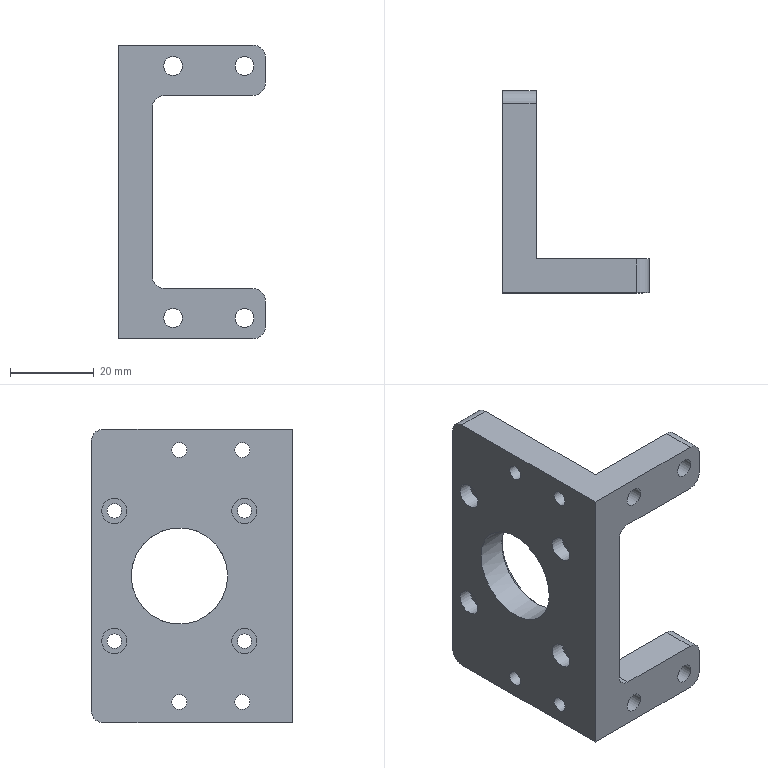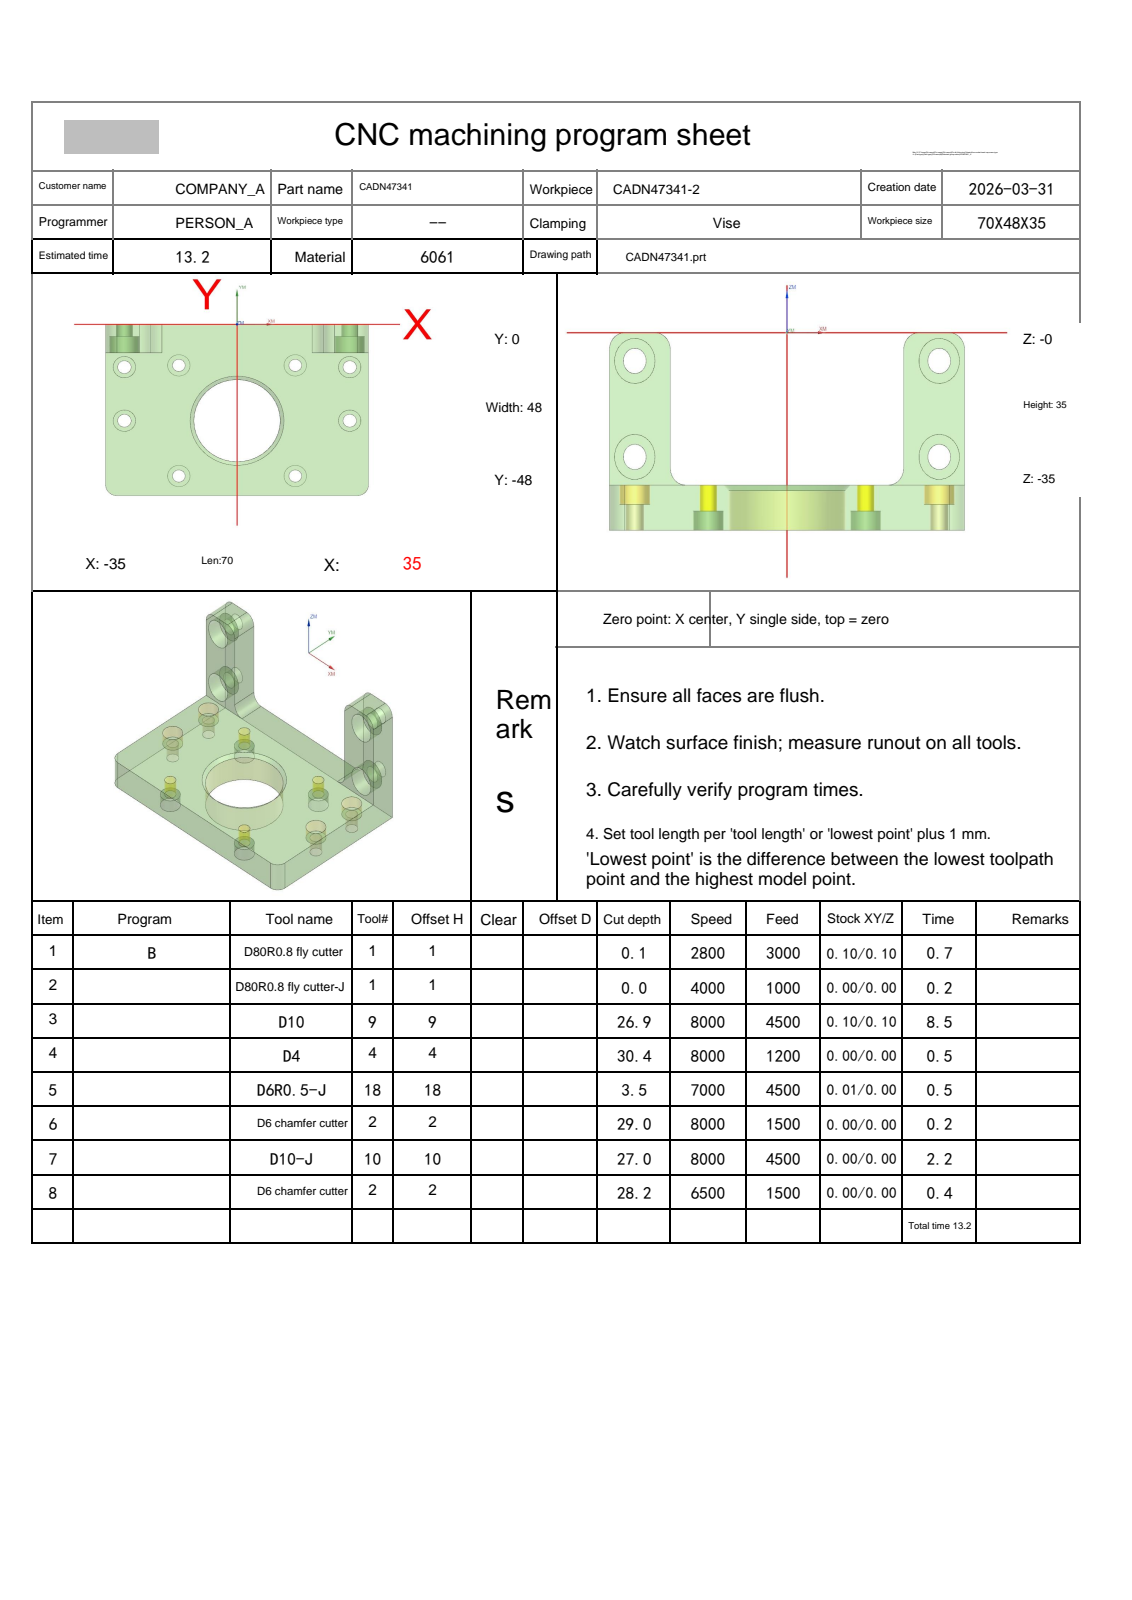NC program | NX | posted by the shop | part box 35 x 48 x 70 mm
Lines 8149 to 9805 of 13995:
N4 T04 M06
(D4  D=4. R=0. H=04 ce=0.07 di=0.00)
G00 G90 G54 X-30. Y-27. M03 S8000
G43 H04 Z20.
M08
Z-26.7
G03 X-30.465 Y-27.465 I0.0 J-.465 F1200.
X-30. Y-27.93 I.465 J0.0
X-30. Y-27.93 Z-26.9 I0.0 J.93
X-30. Y-27.93 Z-27.1 I0.0 J.93
X-30. Y-27.93 Z-27.3 I0.0 J.93
X-30. Y-27.93 Z-27.5 I0.0 J.93
X-30. Y-27.93 Z-27.7 I0.0 J.93
X-30. Y-27.93 Z-27.9 I0.0 J.93
X-30. Y-27.93 Z-28.1 I0.0 J.93
X-30. Y-27.93 Z-28.3 I0.0 J.93
X-30. Y-27.93 Z-28.5 I0.0 J.93
X-30. Y-27.93 Z-28.7 I0.0 J.93
X-30. Y-27.93 Z-28.9 I0.0 J.93
X-30. Y-27.93 Z-29.1 I0.0 J.93
X-30. Y-27.93 Z-29.3 I0.0 J.93
X-30. Y-27.93 Z-29.5 I0.0 J.93
X-30. Y-27.93 Z-29.7 I0.0 J.93
X-30. Y-27.93 Z-29.9 I0.0 J.93
X-30. Y-27.93 Z-30.1 I0.0 J.93
X-30. Y-27.93 Z-30.3 I0.0 J.93
X-30. Y-26.07 Z-30.4 I0.0 J.93
X-30.93 Y-27. I0.0 J-.93
X-30. Y-27.93 I.93 J0.0
X-29.07 Y-27. I0.0 J.93
X-30. Y-26.07 I-.93 J0.0
X-30.465 Y-26.535 I0.0 J-.465
X-30. Y-27. I.465 J0.0
G00 Z20.
Y-12.
Z-26.7
G03 X-30.465 Y-12.465 I0.0 J-.465
X-30. Y-12.93 I.465 J0.0
X-30. Y-12.93 Z-26.9 I0.0 J.93
X-30. Y-12.93 Z-27.1 I0.0 J.93
X-30. Y-12.93 Z-27.3 I0.0 J.93
X-30. Y-12.93 Z-27.5 I0.0 J.93
X-30. Y-12.93 Z-27.7 I0.0 J.93
X-30. Y-12.93 Z-27.9 I0.0 J.93
X-30. Y-12.93 Z-28.1 I0.0 J.93
X-30. Y-12.93 Z-28.3 I0.0 J.93
X-30. Y-12.93 Z-28.5 I0.0 J.93
X-30. Y-12.93 Z-28.7 I0.0 J.93
X-30. Y-12.93 Z-28.9 I0.0 J.93
X-30. Y-12.93 Z-29.1 I0.0 J.93
X-30. Y-12.93 Z-29.3 I0.0 J.93
X-30. Y-12.93 Z-29.5 I0.0 J.93
X-30. Y-12.93 Z-29.7 I0.0 J.93
X-30. Y-12.93 Z-29.9 I0.0 J.93
X-30. Y-12.93 Z-30.1 I0.0 J.93
X-30. Y-12.93 Z-30.3 I0.0 J.93
X-30. Y-11.07 Z-30.4 I0.0 J.93
X-30.93 Y-12. I0.0 J-.93
X-30. Y-12.93 I.93 J0.0
X-29.07 Y-12. I0.0 J.93
X-30. Y-11.07 I-.93 J0.0
X-30.465 Y-11.535 I0.0 J-.465
X-30. Y-12. I.465 J0.0
G00 Z20.
X30.
Z-26.7
G03 X29.535 Y-12.465 I0.0 J-.465
X30. Y-12.93 I.465 J0.0
X30. Y-12.93 Z-26.9 I0.0 J.93
X30. Y-12.93 Z-27.1 I0.0 J.93
X30. Y-12.93 Z-27.3 I0.0 J.93
X30. Y-12.93 Z-27.5 I0.0 J.93
X30. Y-12.93 Z-27.7 I0.0 J.93
X30. Y-12.93 Z-27.9 I0.0 J.93
X30. Y-12.93 Z-28.1 I0.0 J.93
X30. Y-12.93 Z-28.3 I0.0 J.93
X30. Y-12.93 Z-28.5 I0.0 J.93
X30. Y-12.93 Z-28.7 I0.0 J.93
X30. Y-12.93 Z-28.9 I0.0 J.93
X30. Y-12.93 Z-29.1 I0.0 J.93
X30. Y-12.93 Z-29.3 I0.0 J.93
X30. Y-12.93 Z-29.5 I0.0 J.93
X30. Y-12.93 Z-29.7 I0.0 J.93
X30. Y-12.93 Z-29.9 I0.0 J.93
X30. Y-12.93 Z-30.1 I0.0 J.93
X30. Y-12.93 Z-30.3 I0.0 J.93
X30. Y-11.07 Z-30.4 I0.0 J.93
X29.07 Y-12. I0.0 J-.93
X30. Y-12.93 I.93 J0.0
X30.93 Y-12. I0.0 J.93
X30. Y-11.07 I-.93 J0.0
X29.535 Y-11.535 I0.0 J-.465
X30. Y-12. I.465 J0.0
G00 Z20.
Y-27.
Z-26.7
G03 X29.535 Y-27.465 I0.0 J-.465
X30. Y-27.93 I.465 J0.0
X30. Y-27.93 Z-26.9 I0.0 J.93
X30. Y-27.93 Z-27.1 I0.0 J.93
X30. Y-27.93 Z-27.3 I0.0 J.93
X30. Y-27.93 Z-27.5 I0.0 J.93
X30. Y-27.93 Z-27.7 I0.0 J.93
X30. Y-27.93 Z-27.9 I0.0 J.93
X30. Y-27.93 Z-28.1 I0.0 J.93
X30. Y-27.93 Z-28.3 I0.0 J.93
X30. Y-27.93 Z-28.5 I0.0 J.93
X30. Y-27.93 Z-28.7 I0.0 J.93
X30. Y-27.93 Z-28.9 I0.0 J.93
X30. Y-27.93 Z-29.1 I0.0 J.93
X30. Y-27.93 Z-29.3 I0.0 J.93
X30. Y-27.93 Z-29.5 I0.0 J.93
X30. Y-27.93 Z-29.7 I0.0 J.93
X30. Y-27.93 Z-29.9 I0.0 J.93
X30. Y-27.93 Z-30.1 I0.0 J.93
X30. Y-27.93 Z-30.3 I0.0 J.93
X30. Y-26.07 Z-30.4 I0.0 J.93
X29.07 Y-27. I0.0 J-.93
X30. Y-27.93 I.93 J0.0
X30.93 Y-27. I0.0 J.93
X30. Y-26.07 I-.93 J0.0
X29.535 Y-26.535 I0.0 J-.465
X30. Y-27. I.465 J0.0
G00 Z20.
G00 G90 X-30. Y-27. M03 S8000
Z20.
Z-30.4
G01 X-30.272 Y-27.568 F600.
X-30.302 Y-27.698
G03 X-30. Y-28. I.302 J0.0
X-29. Y-27. I0.0 J1.
X-30. Y-26. I-1. J0.0
X-31. Y-27. I0.0 J-1.
X-30. Y-28. I1. J0.0
X-29.521 Y-27.878 I0.0 J1.
X-29.364 Y-27.613 I-.145 J.265
X-29.489 Y-27.368 I-.302 J0.0
G01 X-30. Y-27.
G00 Z20.
Y-12.
Z-30.4
G01 X-30.272 Y-12.568
X-30.302 Y-12.698
G03 X-30. Y-13. I.302 J0.0
X-29. Y-12. I0.0 J1.
X-30. Y-11. I-1. J0.0
X-31. Y-12. I0.0 J-1.
X-30. Y-13. I1. J0.0
X-29.521 Y-12.878 I0.0 J1.
X-29.364 Y-12.613 I-.145 J.265
X-29.489 Y-12.368 I-.302 J0.0
G01 X-30. Y-12.
G00 Z20.
X30.
Z-30.4
G01 X29.728 Y-12.568
X29.698 Y-12.698
G03 X30. Y-13. I.302 J0.0
X31. Y-12. I0.0 J1.
X30. Y-11. I-1. J0.0
X29. Y-12. I0.0 J-1.
X30. Y-13. I1. J0.0
X30.479 Y-12.878 I0.0 J1.
X30.636 Y-12.613 I-.145 J.265
X30.511 Y-12.368 I-.302 J0.0
G01 X30. Y-12.
G00 Z20.
Y-27.
Z-30.4
G01 X29.728 Y-27.568
X29.698 Y-27.698
G03 X30. Y-28. I.302 J0.0
X31. Y-27. I0.0 J1.
X30. Y-26. I-1. J0.0
X29. Y-27. I0.0 J-1.
X30. Y-28. I1. J0.0
X30.479 Y-27.878 I0.0 J1.
X30.636 Y-27.613 I-.145 J.265
X30.511 Y-27.368 I-.302 J0.0
G01 X30. Y-27.
G00 Z20.
G91 G28 Z0.0
M05
M09
G91 G28 Z0.0
M01
N5 T18 M06
(D6R0.5-J  D=6. R=0.5 H=18 ce=0.01 di=0.00)
G00 G90 G54 X34.089 Y6.274 M03 S7000
G43 H18 Z14.5
M08
Z.494
G01 Z-.006 F4500.
X34.596 Y1.122
X34.707 Y0.0
Y-8.
X34.606 Y-8.912
X34.546 Y-9.111
X34.648 Y-9.103 Z-.012
X34.682 Y-8.912
X34.794 Y-8.
Y0.0
X34.687 Y1.105
X34.742 Y1.101 Z-.015
X34.77 Y1.1 Z-.019
X34.877 Y0.0
Y-8.
X34.764 Y-8.912
X34.757 Y-9.1
X34.805 Z-.024
X34.838 Z-.03
X34.844 Y-8.912
X34.964 Y-8.
Y0.0
X34.848 Y1.1
X34.911 Z-.036
X34.942 Z-.042
X35.049 Y0.0
Y-8.
X34.939 Y-8.912
X34.935 Y-9.1
X35. Z-.049
X35.053 Z-.057
X35.056 Y-8.912
X35.138 Y-8.
Y0.0
X35.126 Y.048
X35.057 Y1.1
X35.109 Z-.066
X35.148 Z-.075
X35.208 Y.048
X35.228 Y0.0
Y-8.
X35.148 Y-8.912
X35.146 Y-9.1
X35.207 Z-.085
X35.241 Z-.095
X35.32 Y-8.
Y0.0
X35.302 Y.048
X35.243 Y1.1
X35.306 Z-.107
X35.351 Z-.118
X35.413 Y0.0
Y-8.
X35.349 Y-9.1
X35.406 Z-.132
X35.453 Z-.145
X35.456 Y-8.912
X35.506 Y-8.
Y0.0
X35.494 Y.048
X35.455 Y1.1
X35.504 Z-.159
X35.542 Z-.174
X35.583 Y.048
X35.598 Y0.0
Y-8.
X35.54 Y-9.1
X35.6 Z-.189
X35.635 Z-.205
X35.691 Y-8.
Y0.0
X35.68 Y.048
X35.637 Y1.1
X35.696 Z-.222
X35.74 Z-.24
X35.783 Y0.0
Y-8.
X35.741 Y-8.912
X35.738 Y-9.1
X35.791 Z-.258
X35.827 Z-.277
X35.874 Y-8.
Y0.0
X35.863 Y.048
X35.829 Y1.1
X35.883 Z-.297
X35.916 Z-.316
X35.964 Y0.0
Y-8.
X35.915 Y-9.1
X35.976 Z-.338
X36.008 Z-.359
X36.054 Y-8.
Y0.0
X36.01 Y1.1
X36.067 Z-.381
X36.109 Z-.404
X36.138 Y.048
X36.142 Y0.0
Y-8.
X36.108 Y-9.1
X36.155 Z-.427
X36.196 Z-.451
X36.229 Y-8.
Y0.0
X36.218 Y.048
X36.197 Y1.1
X36.244 Y1.101 Z-.476
X36.287 Z-.501
X36.304 Y.048
X36.315 Y0.0
Y-8.
X36.287 Y-9.1
X36.33 Z-.527
X36.369 Z-.554
X36.399 Y-8.
Y0.0
X36.393 Y.048
X36.37 Y1.1
X36.415 Z-.581
X36.456 Z-.609
X36.482 Y0.0
Y-8.
X36.454 Y-9.1
X36.499 Z-.637
X36.529 Z-.666
X36.564 Y-8.
Y0.0
X36.531 Y1.1
X36.58 Z-.696
X36.609 Z-.725
X36.632 Y.048
X36.643 Y0.0
Y-8.
X36.61 Y-8.912
X36.607 Y-9.1
X36.659 Z-.756
X36.688 Z-.787
X36.722 Y-8.
Y0.0
X36.69 Y1.1
X36.737 Z-.819
X36.774 Z-.851
X36.793 Y.171
X36.798 Y0.0
Y-8.
X36.772 Y-9.1
X36.814 Z-.884
X36.848 Z-.918
X36.872 Y-8.
Y0.0
X36.849 Y1.1
X36.888 Z-.952
X36.924 Z-.986
X36.945 Y0.0
Y-8.
X36.923 Y-9.1
X36.96 Z-1.021
X36.994 Z-1.056
X37.016 Y-8.
Y0.0
X36.995 Y1.1
X37.031 Z-1.093
X37.063 Z-1.129
X37.085 Y0.0
Y-8.
X37.061 Y-9.1
X37.098 Z-1.166
X37.13 Z-1.203
X37.151 Y-8.
Y0.0
X37.132 Y1.1
X37.167 Z-1.241
X37.193 Z-1.28
X37.216 Y0.0
Y-8.
X37.194 Y-8.912
X37.192 Y-9.1
X37.229 Z-1.319
X37.255 Z-1.358
X37.257 Y-8.912
X37.278 Y-8.
Y0.0
X37.256 Y1.1
X37.29 Z-1.398
X37.318 Z-1.438
X37.335 Y.048
X37.338 Y0.0
Y-8.
X37.319 Y-8.912
X37.317 Y-9.1
X37.349 Z-1.478
X37.372 Z-1.519
X37.371 Y-8.937
G02 X37.396 Y-8. I18.046 J0.0
G01 Y0.0
X37.391 Y.048
X37.373 Y1.1
X37.407 Z-1.561
X37.43 Z-1.602
X37.448 Y.048
X37.451 Y0.0
Y-8.
G03 X37.428 Y-8.963 I20.006 J-.963
G01 Y-9.1
X37.46 Z-1.645
X37.484 Z-1.687
Y-8.956
G02 X37.504 Y-8. I22.687 J0.0
G01 Y0.0
X37.501 Y.048
X37.482 Y1.199
X37.525 Y1.254 Z-1.773
G03 X37.554 Y0.0 I77.48 J1.165
G01 Y-8.
G03 X37.531 Y-8.927 I18.186 J-.927
G01 X37.532 Y-9.1
X37.563 Z-1.817
X37.58 Z-1.861
X37.579 Y-8.943
G02 X37.603 Y-8. I19.076 J0.0
G01 Y0.0
G02 X37.573 Y1.254 I126.284 J3.571
G01 X37.605 Z-1.905
X37.622 Z-1.95
G02 X37.648 Y0.0 I-513.452 J-11.351
G01 Y-8.
G03 X37.629 Y-9.028 I27.301 J-1.028
G01 Y-9.1
X37.654 Z-1.995
X37.671 Z-2.04
X37.67 Y-8.92
G02 X37.691 Y-8. I19.851 J0.0
G01 Y0.0
G02 X37.666 Y1.254 I55.734 J1.76
G01 X37.691 Z-2.086
X37.703 Z-2.132
G03 X37.731 Y0.0 I31.796 J.092
G01 Y-8.
G03 X37.706 Y-8.904 I15.853 J-.904
G01 X37.707 Y-9.1
X37.735 Z-2.178
X37.744 Z-2.224
X37.743 Y-8.917
G02 X37.769 Y-8. I15.88 J0.0
G01 Y0.0
G02 X37.741 Y1.21 I25.837 J1.21
G01 Y1.254
X37.768 Z-2.271
X37.776 Z-2.318
G03 X37.804 Y0.0 I68.546 J.918
G01 Y-8.
G03 X37.781 Y-8.97 I19.819 J-.97
G01 Y-9.1
X37.804 Z-2.365
X37.821 Z-2.412
G02 X37.82 Y-8.869 I22.498 J.231
X37.837 Y-8. I22.499 J0.0
G01 Y0.0
X37.834 Y.048
X37.821 Y1.1
X37.836 Z-2.46
X37.85 Z-2.508
G03 X37.847 Y.791 I15.845 J-.309
X37.866 Y0.0 I15.848 J0.0
G01 Y-8.
G03 X37.845 Y-8.923 I19.458 J-.923
G01 Y-9.092
X37.871 Y-9.084 Z-2.604
Y-8.924
G02 X37.893 Y-8. I18.828 J0.0
G01 Y0.0
G02 X37.873 Y.741 I13.709 J.741
X37.878 Y1.102 I13.729 J0.0
G01 X37.892 Y1.101 Z-2.653
X37.902 Z-2.701
G03 X37.9 Y.82 I18.924 J-.281
X37.918 Y0.0 I18.926 J0.0
G01 Y-8.
G03 X37.898 Y-8.975 I23.649 J-.975
G01 Y-9.076
X37.921 Y-9.067 Z-2.799
Y-8.923
G02 X37.939 Y-8. I23.129 J0.0
G01 Y0.0
G02 X37.922 Y.854 I21.386 J.854
X37.923 Y1.1 I21.403 J0.0
G01 X37.93 Z-2.848
X37.945 Z-2.897
G03 X37.941 Y.744 I16.614 J-.356
X37.958 Y0.0 I16.618 J0.0
G01 Y-8.
G03 X37.939 Y-8.93 I22.724 J-.93
G01 Y-9.059
X37.957 Y-9.051 Z-2.996
Y-8.952
G02 X37.974 Y-8. I27.373 J0.0
G01 Y0.0
X37.958 Y1.095
X37.962 Z-3.046
X37.971 Y1.096 Z-3.095
X37.987 Y0.0
Y-8.
X37.974 Y-8.912
X37.972 Y-9.042
X37.986 Y-9.034 Z-3.195
X37.997 Y-8.
Y0.0
X37.992 Y.048
X37.981 Y1.096
X37.989 Y1.097 Z-3.271
X37.997 Y.048
X38.003 Y0.0
Y-8.
G03 X37.991 Y-8.832 I30.152 J-.832
G01 X37.992 Y-9.027
X37.998 Y-9.02 Z-3.347
X38.007 Y-8.
Y0.0
X38.001 Y.048
X37.996 Y1.097
X38.003 Y1.098 Z-3.424
X38.006 Y.048
X38.009 Y0.0
Y-8.
X38.004 Y-9.014
X38.009 Y-9.007 Z-3.5
X38.01 Y-8.912
Y-8.
Y0.0
Y1.098
G00 Z14.5
X23.1 Y-13.856
Z.494
G01 Z-.006
X23.4 Y-9.1
X23.399 Y-8.912
X23.293 Y-8.
Y0.0
G03 X23.405 Y.947 I-3.948 J.947
G01 X23.402 Y1.1
X23.352 Z-.009
X23.344 Z-.012
X23.345 Y1.025
G02 X23.206 Y0.0 I-3.853 J0.0
G01 Y-8.
X23.338 Y-8.912
X23.34 Y-9.1
X23.261 Z-.019
X23.259 Y-8.912
X23.123 Y-8.
Y0.0
X23.269 Y1.1
X23.194 Z-.024
X23.17 Z-.03
X23.036 Y0.0
Y-8.
X23.158 Y-9.1
X23.089 Z-.036
X23.054 Z-.042
X23.053 Y-8.912
X22.951 Y-8.
Y0.0
X22.976 Y.048
X23.063 Y1.1
X23. Z-.049
X22.974 Z-.057
X22.887 Y.048
X22.862 Y0.0
Y-8.
X22.967 Y-8.912
X22.969 Y-9.1
X22.889 Z-.066
X22.869 Z-.075
X22.866 Y-8.912
X22.772 Y-8.
Y0.0
X22.781 Y.048
X22.869 Y1.1
X22.794 Z-.085
X22.75 Z-.095
X22.69 Y.048
X22.68 Y0.0
Y-8.
X22.749 Y-8.912
X22.752 Y-9.1
X22.694 Z-.107
X22.662 Z-.118
X22.587 Y-8.
Y0.0
X22.661 Y1.1
X22.592 Z-.132
X22.565 Z-.145
X22.494 Y0.0
Y-8.
X22.567 Y-9.1
X22.496 Z-.159
X22.461 Z-.174
X22.459 Y-8.912
X22.402 Y-8.
Y0.0
X22.46 Y1.1
X22.4 Z-.189
X22.359 Z-.205
X22.319 Y.048
X22.309 Y0.0
Y-8.
X22.36 Y-9.1
X22.303 Z-.222
X22.271 Z-.24
X22.217 Y-8.
Y0.0
X22.231 Y.048
X22.27 Y1.1
X22.209 Z-.258
X22.174 Z-.277
X22.136 Y.048
X22.126 Y0.0
Y-8.
X22.175 Y-9.1
X22.117 Z-.297
X22.072 Z-.316
X22.07 Y-8.912
X22.036 Y-8.
Y0.0
X22.071 Y1.1
X22.024 Z-.338
X21.985 Z-.359
X21.957 Y.048
X21.946 Y0.0
Y-8.
X21.986 Y-9.1
X21.933 Z-.381
X21.9 Z-.404
X21.858 Y-8.
Y0.0
X21.87 Y.048
X21.899 Y1.1
X21.845 Z-.427
X21.808 Z-.451
X21.778 Y.048
X21.771 Y0.0
Y-8.
X21.81 Y-9.1
X21.757 Z-.476
X21.714 Z-.501
X21.685 Y-8.
Y0.0
X21.712 Y1.1
X21.67 Z-.527
X21.635 Z-.554
X21.601 Y0.0
Y-8.
X21.636 Y-9.1
X21.585 Z-.581
X21.556 Z-.609
X21.554 Y-8.912
X21.518 Y-8.
Y0.0
X21.554 Y1.1
X21.501 Z-.637
X21.47 Z-.666
X21.436 Y0.0
Y-8.
X21.472 Y-9.1
X21.42 Z-.696
X21.385 Z-.725
X21.357 Y-8.
Y0.0
X21.384 Y1.1
X21.341 Z-.756
X21.309 Z-.787
X21.282 Y.048
X21.278 Y0.0
Y-8.
X21.308 Y-8.912
X21.31 Y-9.1
X21.262 Z-.819
X21.236 Z-.851
X21.234 Y-8.912
X21.202 Y-8.
Y0.0
G03 X21.237 Y.905 I-11.878 J.905
G01 X21.235 Y1.1
X21.186 Z-.884
X21.159 Z-.918
X21.131 Y.048
X21.128 Y0.0
Y-8.
X21.158 Y-8.912
X21.16 Y-9.1
X21.112 Z-.952
X21.081 Z-.986
X21.055 Y-8.
Y0.0
X21.08 Y1.1
X21.04 Z-1.021
X21.004 Z-1.056
X20.984 Y0.0
Y-8.
X21.005 Y-9.1
X20.969 Z-1.093
X20.938 Z-1.129
X20.915 Y-8.
Y0.0
X20.937 Y1.1
X20.902 Z-1.166
X20.868 Z-1.203
X20.849 Y0.0
Y-8.
X20.87 Y-9.1
X20.835 Z-1.241
X20.807 Z-1.28
X20.805 Y-8.912
X20.784 Y-8.
Y0.0
X20.806 Y1.1
X20.771 Z-1.319
X20.744 Z-1.358
X20.722 Y0.0
Y-8.
X20.743 Y-8.912
X20.745 Y-9.1
X20.71 Z-1.398
X20.681 Z-1.438
X20.68 Y-8.912
X20.662 Y-8.
Y0.0
X20.68 Y1.1
X20.648 Z-1.478
X20.626 Z-1.519
X20.609 Y.048
X20.604 Y0.0
Y-8.
G02 X20.628 Y-8.94 I-18.759 J-.94
G01 X20.627 Y-9.1
X20.594 Z-1.561
X20.572 Z-1.602
Y-8.956
G03 X20.549 Y-8. I-19.736 J0.0
G01 Y0.0
X20.552 Y.048
X20.57 Y1.1
X20.54 Y1.101 Z-1.645
X20.514 Z-1.687
X20.498 Y.048
X20.496 Y0.0
Y-8.
X20.513 Y-8.912
X20.515 Y-9.1
X20.485 Z-1.73
X20.467 Z-1.773
X20.468 Y-8.935
G03 X20.446 Y-8. I-19.449 J0.0
G01 Y0.0
X20.451 Y.048
X20.466 Y1.1
X20.438 Z-1.817
X20.419 Z-1.861
X20.403 Y.048
X20.397 Y0.0
Y-8.
G02 X20.42 Y-8.942 I-19.368 J-.942
G01 Y-9.1
X20.391 Z-1.905
X20.371 Z-1.95
G03 X20.352 Y-8. I-115.458 J-1.499
G01 Y0.0
X20.354 Y.048
X20.37 Y1.1
X20.347 Z-1.995
X20.324 Z-2.04
G02 X20.326 Y.872 I-22.983 J-.227
X20.309 Y0.0 I-22.984 J0.0
G01 Y-8.
G02 X20.326 Y-8.946 I-25.592 J-.946
G01 Y-9.1
X20.303 Z-2.086
X20.287 Z-2.132
G03 X20.289 Y-8.886 I-19.68 J.214
X20.269 Y-8. I-19.681 J0.0
G01 Y0.0
G03 X20.288 Y.808 I-16.637 J.808
X20.286 Y1.1 I-16.657 J0.0
G01 X20.265 Z-2.178
X20.247 Z-2.224
G02 X20.251 Y.778 I-15.101 J-.322
X20.231 Y0.0 I-15.104 J0.0
G01 Y-8.
G02 X20.251 Y-8.815 I-16.022 J-.815
X20.249 Y-9.1 I-16.043 J0.0
G01 X20.229 Z-2.271
X20.216 Z-2.318
X20.217 Y-8.905
G03 X20.196 Y-8. I-19.286 J0.0
G01 Y0.0
G03 X20.216 Y.827 I-16.483 J.827
X20.214 Y1.1 I-16.504 J0.0
G01 X20.195 Z-2.365
X20.181 Z-2.412
Y.915
G02 X20.163 Y0.0 I-23.204 J0.0
G01 Y-8.
G02 X20.183 Y-9.015 I-26.535 J-1.015
G01 Y-9.101
X20.164 Z-2.46
X20.153 Z-2.508
X20.154 Y-8.937
G03 X20.134 Y-8. I-21.378 J0.0
G01 Y0.0
G03 X20.153 Y.892 I-20.57 J.892
X20.152 Y1.1 I-20.589 J0.0
G01 X20.133 Z-2.556
X20.126 Z-2.604
G02 X20.128 Y.896 I-19.123 J-.205
X20.107 Y0.0 I-19.124 J0.0
G01 Y-8.
G02 X20.129 Y-8.943 I-19.919 J-.943
G01 X20.128 Y-9.101
X20.111 Z-2.653
X20.103 Z-2.701
Y-8.999
G03 X20.082 Y-8. I-24.126 J0.0
G01 Y0.0
G03 X20.102 Y.929 I-22.514 J.929
G01 X20.101 Y1.1
X20.087 Z-2.75
X20.077 Z-2.799
X20.078 Y.902
G02 X20.061 Y0.0 I-24.129 J0.0
G01 Y-8.
G02 X20.079 Y-8.969 I-26.133 J-.969
G01 Y-9.1
X20.07 Y-9.101 Z-2.848
X20.062 Z-2.897
Y-9.066
G03 X20.042 Y-8. I-29.214 J0.0
G01 Y0.0
G03 X20.06 Y.913 I-23.599 J.912
G01 X20.059 Y1.1
X20.052 Z-2.947
X20.041 Y1.101 Z-2.996
X20.03 Y.048
X20.026 Y0.0
Y-8.
X20.045 Y-9.101
X20.035 Y-9.1 Z-3.046
X20.032 Z-3.095
Y-8.992
G03 X20.013 Y-8. I-26.764 J0.0
G01 Y0.0
X20.019 Y.048
X20.029 Y1.1
X20.02 Z-3.145
X20.018 Z-3.195
G02 X20.02 Y.838 I-21.327 J-.262
X20.003 Y0.0 I-21.329 J0.0
G01 Y-8.
X20.021 Y-9.1
X20.013 Z-3.271
X19.998 Y-8.
Y0.0
G03 X20.011 Y.841 I-26.074 J.841
X20.01 Y1.1 I-26.088 J0.0
G01 X20.001 Z-3.347
X19.993 Y0.0
Y-8.
X20.005 Y-9.1
X19.995 Y-9.097 Z-3.424
X19.991 Y-8.
Y0.0
X19.994 Y1.099
X19.99 Y1.098 Z-3.5
Y0.0
Y-8.
Y-8.912
X19.992 Y-9.085
G00 Z14.5
X-23.167 Y5.901
Z.494
G01 Z-.006
X-23.399 Y1.1
X-23.404 Y.914
G03 X-23.293 Y0.0 I3.836 J0.0
G01 Y-8.
X-23.404 Y-9.1
X-23.352 Z-.009
X-23.345 Z-.012
X-23.206 Y-8.
Y0.0
G02 X-23.341 Y.96 I3.347 J.96
G01 X-23.338 Y1.1
X-23.259 Z-.019
X-23.123 Y0.0
Y-8.
X-23.27 Y-9.1
X-23.193 Z-.024
X-23.171 Z-.03
X-23.036 Y-8.
Y0.0
X-23.156 Y1.1
X-23.089 Z-.036
X-23.053 Z-.042
X-22.951 Y0.0
Y-8.
X-23.061 Y-8.912
X-23.064 Y-9.1
X-23. Z-.049
X-22.976 Z-.057
X-22.973 Y-8.912
X-22.862 Y-8.
Y0.0
X-22.968 Y1.1
X-22.89 Z-.066
X-22.867 Z-.075
X-22.772 Y0.0
Y-8.
X-22.872 Y-9.1
X-22.794 Z-.085
X-22.752 Z-.095
X-22.749 Y-8.912
X-22.68 Y-8.
Y0.0
X-22.69 Y.048
X-22.75 Y1.1
X-22.694 Z-.107
X-22.661 Z-.118
X-22.587 Y0.0
Y-8.
X-22.662 Y-9.1
X-22.592 Z-.132
X-22.567 Z-.145
X-22.494 Y-8.
Y0.0
X-22.565 Y1.1
X-22.496 Z-.159
X-22.46 Z-.174
X-22.402 Y0.0
Y-8.
X-22.459 Y-8.912
X-22.461 Y-9.1
X-22.4 Z-.189
X-22.36 Z-.205
X-22.309 Y-8.
Y0.0
X-22.319 Y.048
X-22.359 Y1.1
X-22.303 Z-.222
X-22.27 Z-.24
X-22.231 Y.048
X-22.217 Y0.0
Y-8.
X-22.271 Y-9.1
X-22.209 Z-.258
X-22.175 Z-.277
X-22.126 Y-8.
Y0.0
X-22.136 Y.048
X-22.174 Y1.1
X-22.117 Z-.297
X-22.071 Z-.316
X-22.036 Y0.0
Y-8.
X-22.07 Y-8.912
X-22.072 Y-9.1
X-22.024 Z-.338
X-21.986 Z-.359
X-21.946 Y-8.
Y0.0
X-21.957 Y.048
X-21.985 Y1.1
X-21.933 Z-.381
X-21.899 Z-.404
X-21.87 Y.048
X-21.858 Y0.0
Y-8.
X-21.9 Y-9.1
X-21.845 Z-.427
X-21.81 Z-.451
X-21.771 Y-8.
Y0.0
X-21.778 Y.048
X-21.808 Y1.1
X-21.757 Z-.476
X-21.712 Z-.501
X-21.688 Y.048
X-21.685 Y0.0
Y-8.
X-21.714 Y-9.1
X-21.67 Z-.527
X-21.636 Z-.554
X-21.601 Y-8.
Y0.0
X-21.635 Y1.1
X-21.585 Z-.581
X-21.554 Z-.609
X-21.518 Y0.0
Y-8.
X-21.554 Y-8.912
X-21.556 Y-9.1
X-21.501 Z-.637
X-21.472 Z-.666
X-21.436 Y-8.
Y0.0
X-21.47 Y1.1
X-21.42 Z-.696
X-21.384 Z-.725
X-21.357 Y0.0
Y-8.
X-21.385 Y-9.1
X-21.341 Z-.756
X-21.31 Z-.787
X-21.308 Y-8.912
X-21.278 Y-8.
Y0.0
X-21.282 Y.048
X-21.309 Y1.1
X-21.262 Z-.819
X-21.235 Z-.851
X-21.237 Y.905
G03 X-21.202 Y0.0 I11.913 J0.0
G01 Y-8.
X-21.234 Y-8.912
X-21.236 Y-9.1
X-21.186 Z-.884
X-21.16 Z-.918
X-21.158 Y-8.912
X-21.128 Y-8.
Y0.0
X-21.131 Y.048
X-21.159 Y1.1
X-21.112 Z-.952
X-21.08 Z-.986
X-21.055 Y0.0
Y-8.
X-21.081 Y-9.1
X-21.04 Z-1.021
X-21.005 Z-1.056
X-20.984 Y-8.
Y0.0
X-21.004 Y1.1
X-20.969 Z-1.093
X-20.937 Z-1.129
X-20.915 Y0.0
Y-8.
X-20.938 Y-9.1
X-20.902 Z-1.166
X-20.87 Z-1.203
X-20.849 Y-8.
Y0.0
X-20.868 Y1.1
X-20.835 Z-1.241
X-20.806 Z-1.28
X-20.784 Y0.0
Y-8.
X-20.805 Y-8.912
X-20.807 Y-9.1
X-20.771 Z-1.319
X-20.745 Z-1.358
X-20.743 Y-8.912
X-20.722 Y-8.
Y0.0
X-20.744 Y1.1
X-20.71 Z-1.398
X-20.68 Z-1.438
X-20.662 Y0.0
Y-8.
X-20.68 Y-8.912
X-20.681 Y-9.1
X-20.651 Z-1.478
X-20.627 Z-1.519
X-20.628 Y-8.94
G02 X-20.604 Y-8. I18.782 J0.0
G01 Y0.0
X-20.609 Y.048
X-20.626 Y1.1
X-20.593 Z-1.561
X-20.57 Z-1.602
X-20.552 Y.048
X-20.549 Y0.0
Y-8.
G03 X-20.572 Y-8.956 I19.712 J-.956
G01 Y-9.1
X-20.54 Z-1.645
X-20.515 Z-1.687
X-20.513 Y-8.912
X-20.496 Y-8.
Y0.0
X-20.514 Y1.101
X-20.487 Z-1.73
X-20.466 Y1.1 Z-1.773
X-20.451 Y.048
X-20.446 Y0.0
Y-8.
G03 X-20.468 Y-8.935 I19.427 J-.935
G01 X-20.467 Y-9.1
X-20.438 Z-1.817
X-20.42 Z-1.861
Y-8.942
G02 X-20.397 Y-8. I19.391 J0.0
G01 Y0.0
X-20.403 Y.048
X-20.419 Y1.1
X-20.391 Z-1.905
X-20.37 Z-1.95
X-20.354 Y.048
X-20.352 Y0.0
Y-8.
G03 X-20.372 Y-9.012 I26. J-1.011
G01 X-20.371 Y-9.1
X-20.347 Z-1.995
X-20.326 Z-2.04
Y-8.946
G02 X-20.309 Y-8. I25.61 J0.0
G01 Y0.0
G02 X-20.326 Y.872 I22.968 J.872
X-20.324 Y1.1 I22.984 J0.0
G01 X-20.305 Z-2.086
X-20.286 Z-2.132
G03 X-20.288 Y.808 I16.654 J-.291
X-20.269 Y0.0 I16.657 J0.0
G01 Y-8.
G03 X-20.289 Y-8.886 I19.661 J-.886
X-20.287 Y-9.1 I19.681 J0.0
G01 X-20.265 Z-2.178
X-20.249 Z-2.224
G02 X-20.251 Y-8.815 I16.04 J.285
X-20.231 Y-8. I16.043 J0.0
G01 Y0.0
G02 X-20.251 Y.778 I15.084 J.778
X-20.247 Y1.1 I15.104 J0.0
G01 X-20.229 Z-2.271
X-20.214 Z-2.318
G03 X-20.216 Y.827 I16.501 J-.273
X-20.196 Y0.0 I16.504 J0.0
G01 Y-8.
G03 X-20.217 Y-8.905 I19.264 J-.905
G01 X-20.216 Y-9.1
X-20.196 Z-2.365
X-20.183 Y-9.101 Z-2.412
Y-9.015
G02 X-20.163 Y-8. I26.554 J0.0
G01 Y0.0
G02 X-20.181 Y.915 I23.186 J.915
G01 Y1.1
X-20.164 Z-2.46
X-20.152 Z-2.508
G03 X-20.153 Y.892 I20.588 J-.207
X-20.134 Y0.0 I20.589 J0.0
G01 Y-8.
G03 X-20.154 Y-8.937 I21.357 J-.937
G01 X-20.153 Y-9.1
X-20.136 Y-9.101 Z-2.556
X-20.128 Z-2.604
X-20.129 Y-8.943
G02 X-20.107 Y-8. I19.94 J0.0
G01 Y0.0
G02 X-20.128 Y.896 I19.103 J.896
X-20.126 Y1.1 I19.124 J0.0
G01 X-20.108 Z-2.653
X-20.101 Z-2.701
X-20.102 Y.929
G03 X-20.082 Y0.0 I22.534 J0.0
G01 Y-8.
G03 X-20.103 Y-8.999 I24.104 J-.999
G01 Y-9.101
X-20.087 Z-2.75
X-20.078 Y-9.1 Z-2.799
X-20.079 Y-8.959
G02 X-20.061 Y-8. I25.656 J0.0
G01 Y0.0
G02 X-20.078 Y.913 I24.651 J.913
G01 X-20.077 Y1.1
X-20.07 Z-2.848
X-20.06 Z-2.897
Y.961
G03 X-20.042 Y0.0 I25.672 J0.0
G01 Y-8.
G03 X-20.061 Y-8.998 I26.302 J-.998
G01 Y-9.101
X-20.052 Z-2.947
X-20.044 Z-2.996
Y-9.032
G02 X-20.026 Y-8. I31.146 J0.0
G01 Y0.0
X-20.043 Y1.101
X-20.035 Y1.1 Z-3.046
X-20.03 Z-3.095
X-20.019 Y.048
X-20.013 Y0.0
Y-8.
G03 X-20.031 Y-8.929 I24.034 J-.929
G01 Y-9.1
X-20.025 Z-3.145
X-20.02 Z-3.195
X-20.021 Y-8.978
G02 X-20.003 Y-8. I27.699 J0.0
G01 Y0.0
X-20.008 Y.048
X-20.019 Y1.1
X-20.011 Z-3.271
X-19.998 Y0.0
Y-8.
X-20.012 Y-9.1
X-20.004 Z-3.347
X-19.993 Y-8.
Y0.0
X-20.002 Y1.1
X-19.995 Z-3.424
X-19.992 Y.048
X-19.991 Y0.0
Y-8.
X-19.995 Y-9.095
X-19.992 Y-9.084 Z-3.5
X-19.99 Y-8.912
Y-8.
Y0.0
Y1.099
G00 Z14.5
X-34.545 Y-14.062
Z.494
G01 Z-.006
X-34.606 Y-9.101
X-34.608 Y-8.912
X-34.707 Y-8.
Y0.0
X-34.589 Y1.126
X-34.67 Y1.108 Z-.012
X-34.794 Y0.0
Y-8.
X-34.69 Y-8.912
X-34.688 Y-9.1
X-34.742 Z-.015
X-34.768 Z-.019
X-34.77 Y-8.912
X-34.877 Y-8.
Y0.0
X-34.758 Y1.1
X-34.805 Z-.024
X-34.839 Z-.03
X-34.964 Y0.0
Y-8.
X-34.848 Y-8.912
X-34.846 Y-9.1
X-34.911 Z-.036
X-34.94 Z-.042
X-34.943 Y-8.912
X-35.049 Y-8.
Y0.0
X-35.037 Y.048
X-34.936 Y1.1
X-35. Z-.049
X-35.055 Z-.057
X-35.138 Y0.0
Y-8.
X-35.058 Y-8.912
X-35.055 Y-9.1
X-35.109 Z-.066
X-35.147 Z-.075
X-35.149 Y-8.912
X-35.228 Y-8.
Y0.0
X-35.208 Y.048
X-35.147 Y1.1
X-35.207 Z-.085
X-35.243 Z-.095
X-35.302 Y.048
X-35.32 Y0.0
Y-8.
X-35.242 Y-9.1
X-35.306 Z-.107
X-35.349 Z-.118
X-35.413 Y-8.
Y0.0
X-35.351 Y1.1
X-35.406 Z-.132
X-35.455 Z-.145
X-35.494 Y.048
X-35.506 Y0.0
Y-8.
X-35.456 Y-8.912
X-35.453 Y-9.1
X-35.504 Z-.159
X-35.54 Z-.174
X-35.598 Y-8.
Y0.0
X-35.583 Y.048
X-35.542 Y1.1
X-35.6 Z-.189
X-35.637 Z-.205
X-35.68 Y.048
X-35.691 Y0.0
Y-8.
X-35.635 Y-9.1
X-35.696 Z-.222
X-35.738 Z-.24
X-35.741 Y-8.912
X-35.783 Y-8.
Y0.0
X-35.74 Y1.1
X-35.791 Z-.258
X-35.829 Z-.277
X-35.874 Y0.0
Y-8.
X-35.827 Y-9.1
X-35.883 Z-.297
X-35.915 Z-.316
X-35.964 Y-8.
Y0.0
X-35.916 Y1.1
X-35.976 Z-.338
X-36.01 Z-.359
X-36.054 Y0.0
Y-8.
X-36.008 Y-9.1
X-36.067 Z-.381
X-36.108 Z-.404
X-36.142 Y-8.
Y0.0
X-36.138 Y.048
X-36.109 Y1.1
X-36.155 Z-.427
X-36.197 Z-.451
X-36.218 Y.048
X-36.229 Y0.0
Y-8.
X-36.196 Y-9.1
X-36.248 Z-.476
X-36.287 Z-.501
X-36.315 Y-8.
Y0.0
X-36.304 Y.048
X-36.287 Y1.101
X-36.33 Z-.527
X-36.37 Y1.1 Z-.554
X-36.393 Y.048
X-36.399 Y0.0
Y-8.
X-36.369 Y-9.1
X-36.415 Z-.581
X-36.454 Z-.609
X-36.482 Y-8.
Y0.0
X-36.456 Y1.1
X-36.499 Z-.637
X-36.531 Z-.666
X-36.564 Y0.0
Y-8.
X-36.529 Y-9.1
X-36.58 Z-.696
X-36.607 Z-.725
X-36.61 Y-8.912
X-36.643 Y-8.
Y0.0
X-36.632 Y.048
X-36.609 Y1.1
X-36.659 Z-.756
X-36.69 Z-.787
X-36.722 Y0.0
Y-8.
X-36.688 Y-9.1
X-36.738 Z-.819
X-36.772 Z-.851
X-36.798 Y-8.
Y0.0
X-36.774 Y1.1
X-36.814 Z-.884
X-36.849 Z-.918
X-36.872 Y0.0
Y-8.
X-36.848 Y-9.1
X-36.888 Z-.952
X-36.923 Z-.986
X-36.945 Y-8.
Y0.0
X-36.924 Y1.1
X-36.96 Z-1.021
X-36.995 Z-1.056
X-37.016 Y0.0
Y-8.
X-36.994 Y-9.1
X-37.031 Z-1.093
X-37.061 Z-1.129
X-37.085 Y-8.
Y0.0
X-37.063 Y1.1
X-37.098 Z-1.166
X-37.132 Z-1.203
X-37.151 Y0.0
Y-8.
X-37.13 Y-9.1
X-37.165 Z-1.241
X-37.192 Z-1.28
X-37.194 Y-8.912
X-37.216 Y-8.
Y0.0
X-37.212 Y.048
X-37.193 Y1.1
X-37.229 Z-1.319
X-37.256 Z-1.358
X-37.278 Y0.0
Y-8.
X-37.257 Y-8.912
X-37.255 Y-9.1
X-37.29 Z-1.398
X-37.317 Z-1.438
X-37.319 Y-8.912
X-37.338 Y-8.
Y0.0
X-37.335 Y.048
X-37.318 Y1.1
X-37.349 Z-1.478
X-37.373 Z-1.519
X-37.391 Y.048
X-37.396 Y0.0
Y-8.
G02 X-37.372 Y-9.1 I-71.894 J-2.092
G01 X-37.406 Z-1.561
X-37.428 Z-1.602
Y-8.963
G03 X-37.451 Y-8. I-20.029 J0.0
G01 Y0.0
X-37.448 Y.048
X-37.43 Y1.1
X-37.482 Y1.199 Z-1.687
G02 X-37.504 Y0.0 I-33.752 J.009
G01 Y-8.
G02 X-37.484 Y-8.956 I-22.667 J-.956
G01 Y-9.1
X-37.513 Z-1.73
X-37.532 Z-1.773
X-37.531 Y-8.927
G03 X-37.554 Y-8. I-18.21 J0.0
G01 Y0.0
G03 X-37.525 Y1.254 I-77.451 J2.419
G01 X-37.558 Z-1.817
X-37.573 Z-1.861
G02 X-37.603 Y0.0 I-126.313 J2.317
G01 Y-8.
G02 X-37.579 Y-8.943 I-19.053 J-.943
G01 X-37.58 Y-9.1
X-37.609 Z-1.905
X-37.629 Z-1.95
Y-9.028
G03 X-37.648 Y-8. I-27.32 J0.0
G01 Y0.0
G02 X-37.622 Y1.254 I513.478 J-10.097
G01 X-37.65 Z-1.995
X-37.666 Z-2.04
G02 X-37.691 Y0.0 I-55.759 J.506
G01 Y-8.
G02 X-37.67 Y-8.92 I-19.83 J-.92
G01 X-37.671 Y-9.1
X-37.695 Z-2.086
X-37.707 Z-2.132
X-37.706 Y-8.904
G03 X-37.731 Y-8. I-15.879 J0.0
G01 Y0.0
G03 X-37.703 Y1.254 I-31.767 J1.347
G01 X-37.731 Z-2.178
X-37.741 Z-2.224
Y1.203
G02 X-37.769 Y0.0 I-25.589 J0.0
G01 Y-8.
G02 X-37.743 Y-8.917 I-15.854 J-.917
G01 X-37.744 Y-9.1
X-37.772 Z-2.271
X-37.781 Z-2.318
Y-8.97
G03 X-37.804 Y-8. I-19.843 J0.0
G01 Y0.0
G03 X-37.776 Y1.254 I-68.517 J2.172
G01 X-37.821 Y1.1 Z-2.412
X-37.834 Y.048
X-37.837 Y0.0
Y-8.
G02 X-37.82 Y-8.85 I-21.166 J-.85
X-37.821 Y-9.1 I-21.183 J0.0
G01 X-37.845 Y-9.092 Z-2.508
Y-8.923
G03 X-37.866 Y-8. I-19.48 J0.0
G01 Y0.0
G03 X-37.847 Y.791 I-15.821 J.791
X-37.85 Y1.1 I-15.841 J0.0
G01 X-37.866 Y1.102 Z-2.556
X-37.878 Z-2.604
G02 X-37.873 Y.741 I-13.724 J-.361
X-37.893 Y0.0 I-13.729 J0.0
G01 Y-8.
G02 X-37.871 Y-8.924 I-18.805 J-.924
G01 Y-9.084
X-37.898 Y-9.076 Z-2.701
Y-8.975
G03 X-37.918 Y-8. I-23.669 J0.0
G01 Y0.0
G03 X-37.9 Y.82 I-18.908 J.82
X-37.902 Y1.101 I-18.926 J0.0
G01 X-37.914 Y1.1 Z-2.75
X-37.923 Z-2.799
G02 X-37.922 Y.85 I-21.163 J-.25
X-37.939 Y0.0 I-21.165 J0.0
G01 Y-8.
G02 X-37.921 Y-9.067 I-88.048 J-2.034
G01 X-37.938 Y-9.059 Z-2.897
G03 X-37.958 Y-8. I-67.671 J-.71
G01 Y0.0
G03 X-37.941 Y.741 I-16.299 J.741
X-37.945 Y1.1 I-16.316 J0.0
G01 X-37.959 Y1.095 Z-2.996
X-37.958 Y.878
G02 X-37.974 Y0.0 I-25.514 J0.0
G01 Y-8.
X-37.956 Y-9.051
X-37.968 Y-9.042 Z-3.095
X-37.987 Y-8.
Y0.0
X-37.974 Y1.096
X-37.981 Z-3.145
X-37.986 Y1.097 Z-3.195
X-37.992 Y.048
X-37.997 Y0.0
Y-8.
X-37.98 Y-8.912
X-37.979 Y-9.033
X-37.986 Y-9.027 Z-3.271
X-38.003 Y-8.
Y0.0
X-37.997 Y.048
X-37.992 Y1.097
X-37.998 Z-3.347
X-38.001 Y.048
X-38.007 Y0.0
Y-8.
X-37.994 Y-9.02
X-38.002 Y-9.014 Z-3.424
X-38.009 Y-8.
Y0.0
X-38.006 Y.048
X-38.004 Y1.098
X-38.01 Z-3.5
Y0.0
Y-8.
Y-8.912
X-38.009 Y-9.007
G00 Z14.5
G91 G28 Z0.0
M05
M09
G91 G28 Z0.0
M01
N6 T02 M06
(D6 chamfer cutter  D=6. R=0. H=02 ce=0.00 di=0.00)
G00 G90 G54 X-15.5 Y-42.5 M03 S8000
G43 H02 Z20.
M08
G98 G81 X-15.5 Y-42.5 Z-29. R-24. F1000.
X15.5
Y-11.5
X-15.5
G80
G00 Z20.
G00 G90 X-1.2 Y-35.92 M03 S6500
Z20.
Z-27.2
G01 Z-28.7 F1500.
Y-36.
G03 X0.0 Y-37.2 I1.2 J0.0
G01 X.098
G03 X.781 Y-37.17 I-.098 J10.2
X1.012 Y-37.15 I-.781 J10.17
G01 X1.093 Y-37.141
X1.224 Y-37.126
X1.388 Y-37.105
G03 X6.366 Y-34.97 I-1.388 J10.105
G01 X6.461 Y-34.893
X6.586 Y-34.789
G03 X7.006 Y-34.414 I-6.586 J7.789
X7.226 Y-34.199 I-7.006 J7.414
G01 X7.3 Y-34.124
G03 X7.755 Y-33.626 I-7.3 J7.124
X7.961 Y-33.376 I-7.755 J6.626
X10.119 Y-28.281 I-7.961 J6.376
G01 X10.142 Y-28.083
G03 X10.2 Y-27. I-10.142 J1.083
X0.0 Y-16.8 I-10.2 J0.0
X-10.2 Y-27. I0.0 J-10.2
X0.0 Y-37.2 I10.2 J0.0
G01 X.098
G03 X.4 Y-37.192 I-.098 J10.2
X1.553 Y-35.993 I-.047 J1.199
G01 X1.552 Y-35.946
X-1.2 Y-36.2
G03 X0.0 Y-37.4 I1.2 J0.0
G01 X.099
G03 X.796 Y-37.37 I-.099 J10.4
X1.032 Y-37.349 I-.796 J10.369
G01 X1.114 Y-37.34
G03 X1.415 Y-37.303 I-1.114 J10.34
X6.491 Y-35.126 I-1.415 J10.303
G01 X6.588 Y-35.048
X6.715 Y-34.941
G03 X7.143 Y-34.559 I-6.715 J7.941
X7.368 Y-34.34 I-7.143 J7.559
X7.907 Y-33.756 I-7.368 J7.34
X8.117 Y-33.501 I-7.907 J6.755
X10.318 Y-28.306 I-8.117 J6.501
X10.341 Y-28.104 I-10.318 J1.306
X10.4 Y-27. I-10.341 J1.104
X0.0 Y-16.6 I-10.4 J0.0
X-10.4 Y-27. I0.0 J-10.4
X0.0 Y-37.4 I10.4 J0.0
G01 X.099
G03 X.4 Y-37.392 I-.099 J10.4
X1.554 Y-36.193 I-.046 J1.199
G01 X1.553 Y-36.147
X-1.2 Y-36.4
G03 X0.0 Y-37.6 I1.2 J0.0
G01 X.101
G03 X1.052 Y-37.548 I-.101 J10.6
G01 X1.136 Y-37.539
G03 X1.442 Y-37.501 I-1.136 J10.539
X6.616 Y-35.282 I-1.442 J10.501
G01 X6.714 Y-35.202
X6.844 Y-35.094
G03 X7.28 Y-34.704 I-6.844 J8.094
X7.509 Y-34.481 I-7.28 J7.704
X8.274 Y-33.626 I-7.509 J7.481
X10.516 Y-28.332 I-8.274 J6.626
X10.54 Y-28.126 I-10.516 J1.332
X10.6 Y-27. I-10.54 J1.126
X0.0 Y-16.4 I-10.6 J0.0
X-10.6 Y-27. I0.0 J-10.6
X0.0 Y-37.6 I10.6 J0.0
G01 X.101
G03 X.4 Y-37.592 I-.101 J10.6
X1.555 Y-36.393 I-.045 J1.199
G01 X1.554 Y-36.348
X-1.2 Y-36.6
G03 X0.0 Y-37.8 I1.2 J0.0
G01 X.103
G03 X1.072 Y-37.747 I-.103 J10.8
G01 X1.157 Y-37.738
G03 X6.74 Y-35.438 I-1.157 J10.738
G01 X6.841 Y-35.357
X6.974 Y-35.247
G03 X8.211 Y-34.015 I-6.974 J8.247
X8.43 Y-33.751 I-8.211 J7.015
X10.714 Y-28.357 I-8.43 J6.751
X10.739 Y-28.147 I-10.714 J1.357
X10.8 Y-27. I-10.739 J1.147
X0.0 Y-16.2 I-10.8 J0.0
X-10.8 Y-27. I0.0 J-10.8
X0.0 Y-37.8 I10.8 J0.0
G01 X.103
G03 X.4 Y-37.793 I-.103 J10.8
X1.555 Y-36.593 I-.044 J1.199
G01 Y-36.549
X1.552 Y-36.474
Z-27.2
G00 Z20.
G91 G28 Z0.0
M05
M09
G91 G28 Z0.0
M01